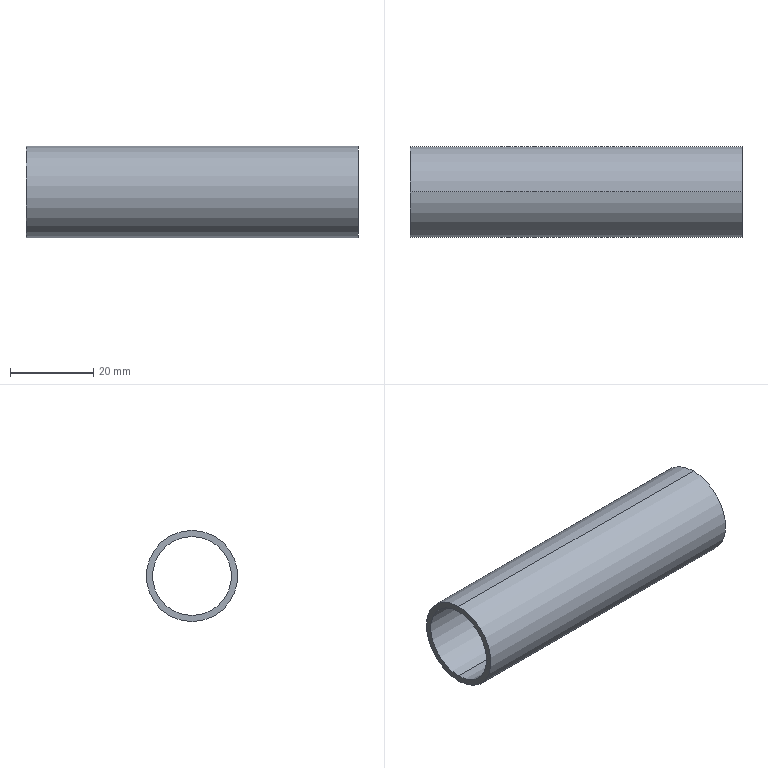Part | STEP file | copper tube 8_default_machined_ | 1 solid | 6 faces | box 80 x 22 x 22 mm | volume 7728 mm3 | cylinder 4 | plane 2 | commonest cylinder face diameters 19 x2 22 x2
STEP:
#1=CARTESIAN_POINT('',(0.,0.,0.));
#2=DIRECTION('',(0.,0.,1.));
#3=DIRECTION('',(1.,0.,0.));
#4=AXIS2_PLACEMENT_3D('',#1,#2,#3);
#5=CARTESIAN_POINT('',(80.,0.,11.));
#6=VERTEX_POINT('',#5);
#7=CARTESIAN_POINT('',(80.,0.,-11.));
#8=VERTEX_POINT('',#7);
#9=CARTESIAN_POINT('',(80.,0.,0.));
#10=DIRECTION('',(-1.,0.,0.));
#11=DIRECTION('',(0.,0.,1.));
#12=AXIS2_PLACEMENT_3D('',#9,#10,#11);
#13=CIRCLE('',#12,11.);
#14=CARTESIAN_POINT('',(80.,0.,0.));
#15=DIRECTION('',(-1.,0.,0.));
#16=DIRECTION('',(0.,0.,1.));
#17=AXIS2_PLACEMENT_3D('',#14,#15,#16);
#18=CYLINDRICAL_SURFACE('',#17,11.);
#19=CARTESIAN_POINT('',(0.,0.));
#20=DIRECTION('',(1.,0.));
#21=VECTOR('',#20,1.);
#22=LINE('',#19,#21);
#23=(GEOMETRIC_REPRESENTATION_CONTEXT(2)PARAMETRIC_REPRESENTATION_CONTEXT()REPRESENTATION_CONTEXT('',''));
#24=DEFINITIONAL_REPRESENTATION('',(#22),#23);
#25=PCURVE('',#18,#24);
#26=CARTESIAN_POINT('',(80.,0.,0.));
#27=DIRECTION('',(1.,0.,0.));
#28=DIRECTION('',(0.,0.,-1.));
#29=AXIS2_PLACEMENT_3D('',#26,#27,#28);
#30=PLANE('',#29);
#31=CARTESIAN_POINT('',(-11.,0.));
#32=CARTESIAN_POINT('',(-11.,19.053));
#33=CARTESIAN_POINT('',(5.5,9.526));
#34=CARTESIAN_POINT('',(22.,0.));
#35=CARTESIAN_POINT('',(5.5,-9.526));
#36=CARTESIAN_POINT('',(-11.,-19.053));
#37=CARTESIAN_POINT('',(-11.,0.));
#38=(BOUNDED_CURVE()B_SPLINE_CURVE(2,(#31,#32,#33,#34,#35,#36,#37),.UNSPECIFIED.,.T.,.F.)B_SPLINE_CURVE_WITH_KNOTS((1,2,2,2,2,1),(-2.094,0.,2.094,4.189,6.283,8.378),.UNSPECIFIED.)CURVE()GEOMETRIC_REPRESENTATION_ITEM()RATIONAL_B_SPLINE_CURVE((1.,0.5,1.,0.5,1.,0.5,1.))REPRESENTATION_ITEM(''));
#39=(GEOMETRIC_REPRESENTATION_CONTEXT(2)PARAMETRIC_REPRESENTATION_CONTEXT()REPRESENTATION_CONTEXT('',''));
#40=DEFINITIONAL_REPRESENTATION('',(#38),#39);
#41=PCURVE('',#30,#40);
#42=SURFACE_CURVE('',#13,(#25,#41),.PCURVE_S1.);
#43=EDGE_CURVE('',#6,#8,#42,.T.);
#44=ORIENTED_EDGE('',*,*,#43,.T.);
#45=CARTESIAN_POINT('',(0.,0.,-11.));
#46=VERTEX_POINT('',#45);
#47=CARTESIAN_POINT('',(80.,0.,-11.));
#48=DIRECTION('',(-1.,0.,0.));
#49=VECTOR('',#48,1.);
#50=LINE('',#47,#49);
#51=CARTESIAN_POINT('',(3.142,0.));
#52=DIRECTION('',(0.,1.));
#53=VECTOR('',#52,1.);
#54=LINE('',#51,#53);
#55=(GEOMETRIC_REPRESENTATION_CONTEXT(2)PARAMETRIC_REPRESENTATION_CONTEXT()REPRESENTATION_CONTEXT('',''));
#56=DEFINITIONAL_REPRESENTATION('',(#54),#55);
#57=PCURVE('',#18,#56);
#58=CARTESIAN_POINT('',(80.,0.,0.));
#59=DIRECTION('',(-1.,0.,0.));
#60=DIRECTION('',(0.,0.,1.));
#61=AXIS2_PLACEMENT_3D('',#58,#59,#60);
#62=CYLINDRICAL_SURFACE('',#61,11.);
#63=CARTESIAN_POINT('',(3.142,0.));
#64=DIRECTION('',(0.,1.));
#65=VECTOR('',#64,1.);
#66=LINE('',#63,#65);
#67=(GEOMETRIC_REPRESENTATION_CONTEXT(2)PARAMETRIC_REPRESENTATION_CONTEXT()REPRESENTATION_CONTEXT('',''));
#68=DEFINITIONAL_REPRESENTATION('',(#66),#67);
#69=PCURVE('',#62,#68);
#70=SURFACE_CURVE('',#50,(#57,#69),.PCURVE_S1.);
#71=EDGE_CURVE('',#8,#46,#70,.T.);
#72=ORIENTED_EDGE('',*,*,#71,.T.);
#73=CARTESIAN_POINT('',(0.,0.,11.));
#74=VERTEX_POINT('',#73);
#75=CARTESIAN_POINT('',(0.,0.,0.));
#76=DIRECTION('',(1.,0.,0.));
#77=DIRECTION('',(0.,0.,1.));
#78=AXIS2_PLACEMENT_3D('',#75,#76,#77);
#79=CIRCLE('',#78,11.);
#80=CARTESIAN_POINT('',(6.283,80.));
#81=DIRECTION('',(-1.,0.));
#82=VECTOR('',#81,1.);
#83=LINE('',#80,#82);
#84=(GEOMETRIC_REPRESENTATION_CONTEXT(2)PARAMETRIC_REPRESENTATION_CONTEXT()REPRESENTATION_CONTEXT('',''));
#85=DEFINITIONAL_REPRESENTATION('',(#83),#84);
#86=PCURVE('',#18,#85);
#87=CARTESIAN_POINT('',(0.,0.,0.));
#88=DIRECTION('',(1.,0.,0.));
#89=DIRECTION('',(0.,0.,-1.));
#90=AXIS2_PLACEMENT_3D('',#87,#88,#89);
#91=PLANE('',#90);
#92=CARTESIAN_POINT('',(0.,0.));
#93=DIRECTION('',(-1.,0.));
#94=AXIS2_PLACEMENT_2D('',#92,#93);
#95=CIRCLE('',#94,11.);
#96=(GEOMETRIC_REPRESENTATION_CONTEXT(2)PARAMETRIC_REPRESENTATION_CONTEXT()REPRESENTATION_CONTEXT('',''));
#97=DEFINITIONAL_REPRESENTATION('',(#95),#96);
#98=PCURVE('',#91,#97);
#99=SURFACE_CURVE('',#79,(#86,#98),.PCURVE_S1.);
#100=EDGE_CURVE('',#46,#74,#99,.T.);
#101=ORIENTED_EDGE('',*,*,#100,.T.);
#102=CARTESIAN_POINT('',(80.,0.,11.));
#103=DIRECTION('',(-1.,0.,0.));
#104=VECTOR('',#103,1.);
#105=LINE('',#102,#104);
#106=CARTESIAN_POINT('',(0.,0.));
#107=DIRECTION('',(0.,1.));
#108=VECTOR('',#107,1.);
#109=LINE('',#106,#108);
#110=(GEOMETRIC_REPRESENTATION_CONTEXT(2)PARAMETRIC_REPRESENTATION_CONTEXT()REPRESENTATION_CONTEXT('',''));
#111=DEFINITIONAL_REPRESENTATION('',(#109),#110);
#112=PCURVE('',#18,#111);
#113=CARTESIAN_POINT('',(6.283,0.));
#114=DIRECTION('',(0.,1.));
#115=VECTOR('',#114,1.);
#116=LINE('',#113,#115);
#117=(GEOMETRIC_REPRESENTATION_CONTEXT(2)PARAMETRIC_REPRESENTATION_CONTEXT()REPRESENTATION_CONTEXT('',''));
#118=DEFINITIONAL_REPRESENTATION('',(#116),#117);
#119=PCURVE('',#62,#118);
#120=SURFACE_CURVE('',#105,(#112,#119),.PCURVE_S1.);
#121=EDGE_CURVE('',#6,#74,#120,.T.);
#122=ORIENTED_EDGE('',*,*,#121,.F.);
#123=EDGE_LOOP('',(#44,#72,#101,#122));
#124=FACE_BOUND('',#123,.T.);
#125=ADVANCED_FACE('',(#124),#18,.T.);
#126=CARTESIAN_POINT('',(80.,0.,9.5));
#127=VERTEX_POINT('',#126);
#128=CARTESIAN_POINT('',(0.,0.,9.5));
#129=VERTEX_POINT('',#128);
#130=CARTESIAN_POINT('',(80.,0.,9.5));
#131=DIRECTION('',(-1.,0.,0.));
#132=VECTOR('',#131,1.);
#133=LINE('',#130,#132);
#134=CARTESIAN_POINT('',(80.,0.,0.));
#135=DIRECTION('',(-1.,0.,0.));
#136=DIRECTION('',(0.,0.,1.));
#137=AXIS2_PLACEMENT_3D('',#134,#135,#136);
#138=CYLINDRICAL_SURFACE('',#137,9.5);
#139=CARTESIAN_POINT('',(6.283,0.));
#140=DIRECTION('',(0.,1.));
#141=VECTOR('',#140,1.);
#142=LINE('',#139,#141);
#143=(GEOMETRIC_REPRESENTATION_CONTEXT(2)PARAMETRIC_REPRESENTATION_CONTEXT()REPRESENTATION_CONTEXT('',''));
#144=DEFINITIONAL_REPRESENTATION('',(#142),#143);
#145=PCURVE('',#138,#144);
#146=CARTESIAN_POINT('',(80.,0.,0.));
#147=DIRECTION('',(-1.,0.,0.));
#148=DIRECTION('',(0.,0.,1.));
#149=AXIS2_PLACEMENT_3D('',#146,#147,#148);
#150=CYLINDRICAL_SURFACE('',#149,9.5);
#151=CARTESIAN_POINT('',(0.,0.));
#152=DIRECTION('',(0.,1.));
#153=VECTOR('',#152,1.);
#154=LINE('',#151,#153);
#155=(GEOMETRIC_REPRESENTATION_CONTEXT(2)PARAMETRIC_REPRESENTATION_CONTEXT()REPRESENTATION_CONTEXT('',''));
#156=DEFINITIONAL_REPRESENTATION('',(#154),#155);
#157=PCURVE('',#150,#156);
#158=SURFACE_CURVE('',#133,(#145,#157),.PCURVE_S1.);
#159=EDGE_CURVE('',#127,#129,#158,.T.);
#160=ORIENTED_EDGE('',*,*,#159,.T.);
#161=CARTESIAN_POINT('',(0.,0.,-9.5));
#162=VERTEX_POINT('',#161);
#163=CARTESIAN_POINT('',(0.,0.,0.));
#164=DIRECTION('',(-1.,0.,0.));
#165=DIRECTION('',(0.,0.,1.));
#166=AXIS2_PLACEMENT_3D('',#163,#164,#165);
#167=CIRCLE('',#166,9.5);
#168=CARTESIAN_POINT('',(0.,80.));
#169=DIRECTION('',(1.,0.));
#170=VECTOR('',#169,1.);
#171=LINE('',#168,#170);
#172=(GEOMETRIC_REPRESENTATION_CONTEXT(2)PARAMETRIC_REPRESENTATION_CONTEXT()REPRESENTATION_CONTEXT('',''));
#173=DEFINITIONAL_REPRESENTATION('',(#171),#172);
#174=PCURVE('',#138,#173);
#175=CARTESIAN_POINT('',(-9.5,0.));
#176=CARTESIAN_POINT('',(-9.5,16.454));
#177=CARTESIAN_POINT('',(4.75,8.227));
#178=CARTESIAN_POINT('',(19.,0.));
#179=CARTESIAN_POINT('',(4.75,-8.227));
#180=CARTESIAN_POINT('',(-9.5,-16.454));
#181=CARTESIAN_POINT('',(-9.5,0.));
#182=(BOUNDED_CURVE()B_SPLINE_CURVE(2,(#175,#176,#177,#178,#179,#180,#181),.UNSPECIFIED.,.T.,.F.)B_SPLINE_CURVE_WITH_KNOTS((1,2,2,2,2,1),(-2.094,0.,2.094,4.189,6.283,8.378),.UNSPECIFIED.)CURVE()GEOMETRIC_REPRESENTATION_ITEM()RATIONAL_B_SPLINE_CURVE((1.,0.5,1.,0.5,1.,0.5,1.))REPRESENTATION_ITEM(''));
#183=(GEOMETRIC_REPRESENTATION_CONTEXT(2)PARAMETRIC_REPRESENTATION_CONTEXT()REPRESENTATION_CONTEXT('',''));
#184=DEFINITIONAL_REPRESENTATION('',(#182),#183);
#185=PCURVE('',#91,#184);
#186=SURFACE_CURVE('',#167,(#174,#185),.PCURVE_S1.);
#187=EDGE_CURVE('',#162,#129,#186,.T.);
#188=ORIENTED_EDGE('',*,*,#187,.F.);
#189=CARTESIAN_POINT('',(80.,0.,-9.5));
#190=VERTEX_POINT('',#189);
#191=CARTESIAN_POINT('',(80.,0.,-9.5));
#192=DIRECTION('',(-1.,0.,0.));
#193=VECTOR('',#192,1.);
#194=LINE('',#191,#193);
#195=CARTESIAN_POINT('',(3.142,0.));
#196=DIRECTION('',(0.,1.));
#197=VECTOR('',#196,1.);
#198=LINE('',#195,#197);
#199=(GEOMETRIC_REPRESENTATION_CONTEXT(2)PARAMETRIC_REPRESENTATION_CONTEXT()REPRESENTATION_CONTEXT('',''));
#200=DEFINITIONAL_REPRESENTATION('',(#198),#199);
#201=PCURVE('',#138,#200);
#202=CARTESIAN_POINT('',(3.142,0.));
#203=DIRECTION('',(0.,1.));
#204=VECTOR('',#203,1.);
#205=LINE('',#202,#204);
#206=(GEOMETRIC_REPRESENTATION_CONTEXT(2)PARAMETRIC_REPRESENTATION_CONTEXT()REPRESENTATION_CONTEXT('',''));
#207=DEFINITIONAL_REPRESENTATION('',(#205),#206);
#208=PCURVE('',#150,#207);
#209=SURFACE_CURVE('',#194,(#201,#208),.PCURVE_S1.);
#210=EDGE_CURVE('',#190,#162,#209,.T.);
#211=ORIENTED_EDGE('',*,*,#210,.F.);
#212=CARTESIAN_POINT('',(80.,0.,0.));
#213=DIRECTION('',(-1.,0.,0.));
#214=DIRECTION('',(0.,0.,1.));
#215=AXIS2_PLACEMENT_3D('',#212,#213,#214);
#216=CIRCLE('',#215,9.5);
#217=CARTESIAN_POINT('',(0.,0.));
#218=DIRECTION('',(1.,0.));
#219=VECTOR('',#218,1.);
#220=LINE('',#217,#219);
#221=(GEOMETRIC_REPRESENTATION_CONTEXT(2)PARAMETRIC_REPRESENTATION_CONTEXT()REPRESENTATION_CONTEXT('',''));
#222=DEFINITIONAL_REPRESENTATION('',(#220),#221);
#223=PCURVE('',#138,#222);
#224=CARTESIAN_POINT('',(-9.5,0.));
#225=CARTESIAN_POINT('',(-9.5,16.454));
#226=CARTESIAN_POINT('',(4.75,8.227));
#227=CARTESIAN_POINT('',(19.,0.));
#228=CARTESIAN_POINT('',(4.75,-8.227));
#229=CARTESIAN_POINT('',(-9.5,-16.454));
#230=CARTESIAN_POINT('',(-9.5,0.));
#231=(BOUNDED_CURVE()B_SPLINE_CURVE(2,(#224,#225,#226,#227,#228,#229,#230),.UNSPECIFIED.,.T.,.F.)B_SPLINE_CURVE_WITH_KNOTS((1,2,2,2,2,1),(-2.094,0.,2.094,4.189,6.283,8.378),.UNSPECIFIED.)CURVE()GEOMETRIC_REPRESENTATION_ITEM()RATIONAL_B_SPLINE_CURVE((1.,0.5,1.,0.5,1.,0.5,1.))REPRESENTATION_ITEM(''));
#232=(GEOMETRIC_REPRESENTATION_CONTEXT(2)PARAMETRIC_REPRESENTATION_CONTEXT()REPRESENTATION_CONTEXT('',''));
#233=DEFINITIONAL_REPRESENTATION('',(#231),#232);
#234=PCURVE('',#30,#233);
#235=SURFACE_CURVE('',#216,(#223,#234),.PCURVE_S1.);
#236=EDGE_CURVE('',#190,#127,#235,.T.);
#237=ORIENTED_EDGE('',*,*,#236,.T.);
#238=EDGE_LOOP('',(#160,#188,#211,#237));
#239=FACE_BOUND('',#238,.F.);
#240=ADVANCED_FACE('',(#239),#138,.F.);
#241=ORIENTED_EDGE('',*,*,#71,.F.);
#242=CARTESIAN_POINT('',(80.,0.,0.));
#243=DIRECTION('',(-1.,0.,0.));
#244=DIRECTION('',(0.,0.,1.));
#245=AXIS2_PLACEMENT_3D('',#242,#243,#244);
#246=CIRCLE('',#245,11.);
#247=CARTESIAN_POINT('',(0.,0.));
#248=DIRECTION('',(1.,0.));
#249=VECTOR('',#248,1.);
#250=LINE('',#247,#249);
#251=(GEOMETRIC_REPRESENTATION_CONTEXT(2)PARAMETRIC_REPRESENTATION_CONTEXT()REPRESENTATION_CONTEXT('',''));
#252=DEFINITIONAL_REPRESENTATION('',(#250),#251);
#253=PCURVE('',#62,#252);
#254=CARTESIAN_POINT('',(-11.,0.));
#255=CARTESIAN_POINT('',(-11.,19.053));
#256=CARTESIAN_POINT('',(5.5,9.526));
#257=CARTESIAN_POINT('',(22.,0.));
#258=CARTESIAN_POINT('',(5.5,-9.526));
#259=CARTESIAN_POINT('',(-11.,-19.053));
#260=CARTESIAN_POINT('',(-11.,0.));
#261=(BOUNDED_CURVE()B_SPLINE_CURVE(2,(#254,#255,#256,#257,#258,#259,#260),.UNSPECIFIED.,.T.,.F.)B_SPLINE_CURVE_WITH_KNOTS((1,2,2,2,2,1),(-2.094,0.,2.094,4.189,6.283,8.378),.UNSPECIFIED.)CURVE()GEOMETRIC_REPRESENTATION_ITEM()RATIONAL_B_SPLINE_CURVE((1.,0.5,1.,0.5,1.,0.5,1.))REPRESENTATION_ITEM(''));
#262=(GEOMETRIC_REPRESENTATION_CONTEXT(2)PARAMETRIC_REPRESENTATION_CONTEXT()REPRESENTATION_CONTEXT('',''));
#263=DEFINITIONAL_REPRESENTATION('',(#261),#262);
#264=PCURVE('',#30,#263);
#265=SURFACE_CURVE('',#246,(#253,#264),.PCURVE_S1.);
#266=EDGE_CURVE('',#8,#6,#265,.T.);
#267=ORIENTED_EDGE('',*,*,#266,.T.);
#268=ORIENTED_EDGE('',*,*,#121,.T.);
#269=CARTESIAN_POINT('',(0.,0.,0.));
#270=DIRECTION('',(1.,0.,0.));
#271=DIRECTION('',(0.,0.,1.));
#272=AXIS2_PLACEMENT_3D('',#269,#270,#271);
#273=CIRCLE('',#272,11.);
#274=CARTESIAN_POINT('',(6.283,80.));
#275=DIRECTION('',(-1.,0.));
#276=VECTOR('',#275,1.);
#277=LINE('',#274,#276);
#278=(GEOMETRIC_REPRESENTATION_CONTEXT(2)PARAMETRIC_REPRESENTATION_CONTEXT()REPRESENTATION_CONTEXT('',''));
#279=DEFINITIONAL_REPRESENTATION('',(#277),#278);
#280=PCURVE('',#62,#279);
#281=CARTESIAN_POINT('',(0.,0.));
#282=DIRECTION('',(-1.,0.));
#283=AXIS2_PLACEMENT_2D('',#281,#282);
#284=CIRCLE('',#283,11.);
#285=(GEOMETRIC_REPRESENTATION_CONTEXT(2)PARAMETRIC_REPRESENTATION_CONTEXT()REPRESENTATION_CONTEXT('',''));
#286=DEFINITIONAL_REPRESENTATION('',(#284),#285);
#287=PCURVE('',#91,#286);
#288=SURFACE_CURVE('',#273,(#280,#287),.PCURVE_S1.);
#289=EDGE_CURVE('',#74,#46,#288,.T.);
#290=ORIENTED_EDGE('',*,*,#289,.T.);
#291=EDGE_LOOP('',(#241,#267,#268,#290));
#292=FACE_BOUND('',#291,.T.);
#293=ADVANCED_FACE('',(#292),#62,.T.);
#294=ORIENTED_EDGE('',*,*,#289,.F.);
#295=ORIENTED_EDGE('',*,*,#100,.F.);
#296=EDGE_LOOP('',(#294,#295));
#297=FACE_BOUND('',#296,.T.);
#298=CARTESIAN_POINT('',(0.,0.,0.));
#299=DIRECTION('',(-1.,0.,0.));
#300=DIRECTION('',(0.,0.,1.));
#301=AXIS2_PLACEMENT_3D('',#298,#299,#300);
#302=CIRCLE('',#301,9.5);
#303=CARTESIAN_POINT('',(-9.5,0.));
#304=CARTESIAN_POINT('',(-9.5,16.454));
#305=CARTESIAN_POINT('',(4.75,8.227));
#306=CARTESIAN_POINT('',(19.,0.));
#307=CARTESIAN_POINT('',(4.75,-8.227));
#308=CARTESIAN_POINT('',(-9.5,-16.454));
#309=CARTESIAN_POINT('',(-9.5,0.));
#310=(BOUNDED_CURVE()B_SPLINE_CURVE(2,(#303,#304,#305,#306,#307,#308,#309),.UNSPECIFIED.,.T.,.F.)B_SPLINE_CURVE_WITH_KNOTS((1,2,2,2,2,1),(-2.094,0.,2.094,4.189,6.283,8.378),.UNSPECIFIED.)CURVE()GEOMETRIC_REPRESENTATION_ITEM()RATIONAL_B_SPLINE_CURVE((1.,0.5,1.,0.5,1.,0.5,1.))REPRESENTATION_ITEM(''));
#311=(GEOMETRIC_REPRESENTATION_CONTEXT(2)PARAMETRIC_REPRESENTATION_CONTEXT()REPRESENTATION_CONTEXT('',''));
#312=DEFINITIONAL_REPRESENTATION('',(#310),#311);
#313=PCURVE('',#91,#312);
#314=CARTESIAN_POINT('',(0.,80.));
#315=DIRECTION('',(1.,0.));
#316=VECTOR('',#315,1.);
#317=LINE('',#314,#316);
#318=(GEOMETRIC_REPRESENTATION_CONTEXT(2)PARAMETRIC_REPRESENTATION_CONTEXT()REPRESENTATION_CONTEXT('',''));
#319=DEFINITIONAL_REPRESENTATION('',(#317),#318);
#320=PCURVE('',#150,#319);
#321=SURFACE_CURVE('',#302,(#313,#320),.PCURVE_S1.);
#322=EDGE_CURVE('',#129,#162,#321,.T.);
#323=ORIENTED_EDGE('',*,*,#322,.F.);
#324=ORIENTED_EDGE('',*,*,#187,.F.);
#325=EDGE_LOOP('',(#323,#324));
#326=FACE_BOUND('',#325,.T.);
#327=ADVANCED_FACE('',(#297,#326),#91,.F.);
#328=ORIENTED_EDGE('',*,*,#43,.F.);
#329=ORIENTED_EDGE('',*,*,#266,.F.);
#330=EDGE_LOOP('',(#328,#329));
#331=FACE_BOUND('',#330,.T.);
#332=CARTESIAN_POINT('',(80.,0.,0.));
#333=DIRECTION('',(-1.,0.,0.));
#334=DIRECTION('',(0.,0.,1.));
#335=AXIS2_PLACEMENT_3D('',#332,#333,#334);
#336=CIRCLE('',#335,9.5);
#337=CARTESIAN_POINT('',(-9.5,0.));
#338=CARTESIAN_POINT('',(-9.5,16.454));
#339=CARTESIAN_POINT('',(4.75,8.227));
#340=CARTESIAN_POINT('',(19.,0.));
#341=CARTESIAN_POINT('',(4.75,-8.227));
#342=CARTESIAN_POINT('',(-9.5,-16.454));
#343=CARTESIAN_POINT('',(-9.5,0.));
#344=(BOUNDED_CURVE()B_SPLINE_CURVE(2,(#337,#338,#339,#340,#341,#342,#343),.UNSPECIFIED.,.T.,.F.)B_SPLINE_CURVE_WITH_KNOTS((1,2,2,2,2,1),(-2.094,0.,2.094,4.189,6.283,8.378),.UNSPECIFIED.)CURVE()GEOMETRIC_REPRESENTATION_ITEM()RATIONAL_B_SPLINE_CURVE((1.,0.5,1.,0.5,1.,0.5,1.))REPRESENTATION_ITEM(''));
#345=(GEOMETRIC_REPRESENTATION_CONTEXT(2)PARAMETRIC_REPRESENTATION_CONTEXT()REPRESENTATION_CONTEXT('',''));
#346=DEFINITIONAL_REPRESENTATION('',(#344),#345);
#347=PCURVE('',#30,#346);
#348=CARTESIAN_POINT('',(0.,0.));
#349=DIRECTION('',(1.,0.));
#350=VECTOR('',#349,1.);
#351=LINE('',#348,#350);
#352=(GEOMETRIC_REPRESENTATION_CONTEXT(2)PARAMETRIC_REPRESENTATION_CONTEXT()REPRESENTATION_CONTEXT('',''));
#353=DEFINITIONAL_REPRESENTATION('',(#351),#352);
#354=PCURVE('',#150,#353);
#355=SURFACE_CURVE('',#336,(#347,#354),.PCURVE_S1.);
#356=EDGE_CURVE('',#127,#190,#355,.T.);
#357=ORIENTED_EDGE('',*,*,#356,.T.);
#358=ORIENTED_EDGE('',*,*,#236,.T.);
#359=EDGE_LOOP('',(#357,#358));
#360=FACE_BOUND('',#359,.T.);
#361=ADVANCED_FACE('',(#331,#360),#30,.T.);
#362=ORIENTED_EDGE('',*,*,#322,.F.);
#363=ORIENTED_EDGE('',*,*,#159,.F.);
#364=ORIENTED_EDGE('',*,*,#356,.T.);
#365=ORIENTED_EDGE('',*,*,#210,.T.);
#366=EDGE_LOOP('',(#362,#363,#364,#365));
#367=FACE_BOUND('',#366,.F.);
#368=ADVANCED_FACE('',(#367),#150,.F.);
#369=CLOSED_SHELL('',(#125,#240,#293,#327,#361,#368));
#370=MANIFOLD_SOLID_BREP('',#369);
#371=(LENGTH_UNIT()NAMED_UNIT(*)SI_UNIT(.MILLI.,.METRE.));
#372=UNCERTAINTY_MEASURE_WITH_UNIT(LENGTH_MEASURE(0.0000001),#371,'','');
#373=(NAMED_UNIT(*)PLANE_ANGLE_UNIT()SI_UNIT($,.RADIAN.));
#374=(NAMED_UNIT(*)SI_UNIT($,.STERADIAN.)SOLID_ANGLE_UNIT());
#375=(GEOMETRIC_REPRESENTATION_CONTEXT(3)GLOBAL_UNCERTAINTY_ASSIGNED_CONTEXT((#372))GLOBAL_UNIT_ASSIGNED_CONTEXT((#371,#373,#374))REPRESENTATION_CONTEXT('',''));
#376=ADVANCED_BREP_SHAPE_REPRESENTATION('',(#4,#370),#375);